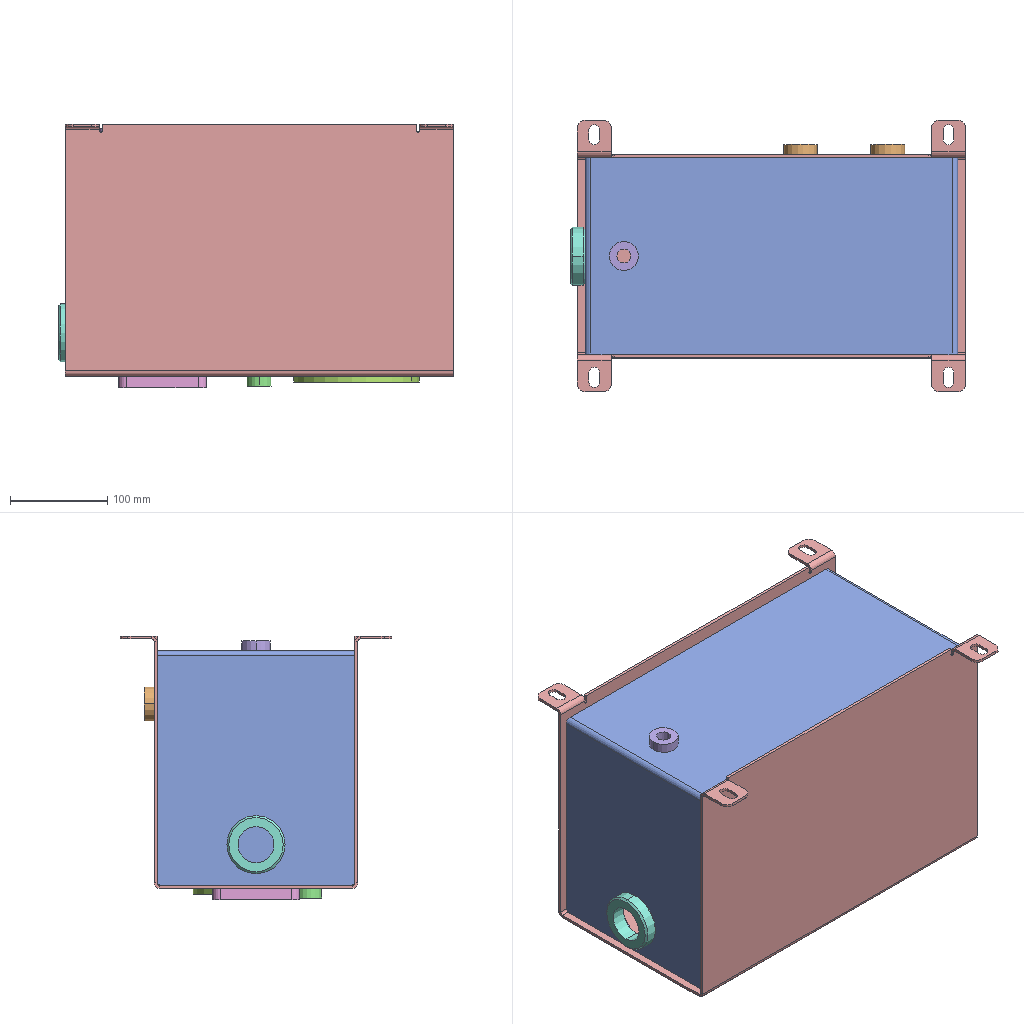Assembly | SolidWorks | 8 different items | 9 placed | box 407 x 280 x 272 mm
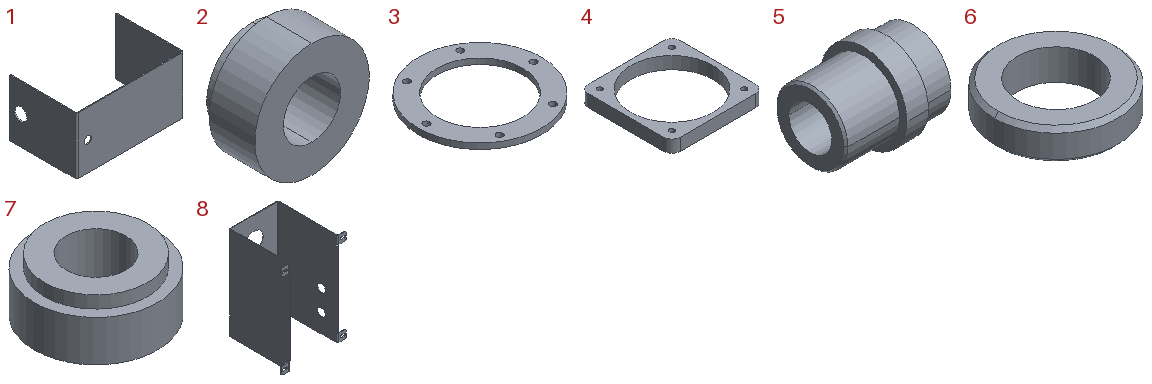Parts list (item | quantity | size | volume | features):
1 | x1 | 384 x 242 x 204 mm | 519134 mm3 | features ICE 2, Fillet 1, FlatPattern 1, SMBaseFlange 1, SheetMetal 1, UnFold 1
2 | x1 | 25 x 13 x 25 mm | 4256 mm3 | features HoleWzd 1, Revolution 1
3 | x1 | 130 x 130 x 6 mm | 40162 mm3 | features FlatPattern 1, HoleWzd 1, SMBaseFlange 1, SheetMetal 1
4 | x1 | 90 x 90 x 12 mm | 35280 mm3 | features FlatPattern 1, HoleWzd 1, SMBaseFlange 1, SheetMetal 1
5 | x2 | 48 x 40 x 40 mm | 30975 mm3 | features HoleWzd 1, ICE 1, Revolution 1
6 | x1 | 60 x 60 x 15 mm | 25107 mm3 | features Chamfer 1, Extrusion 1, HoleWzd 1, ICE 1
7 | x1 | 30 x 30 x 13 mm | 6395 mm3 | features ICE 2, Extrusion 1, HoleWzd 1
8 | x1 | 280 x 260 x 400 mm | 833549 mm3 | features ICE 4, EdgeFlange 1, Fillet 1, FlatPattern 1, SMBaseFlange 1, SheetMetal 1, UnFold 1
Mates (type | each side: item.copy, entity, surface, feature):
Coincident | 8.1 face plane Base-Flange1 | 1.1 face plane Base-Flange1 | 2 times
DistanceDim | 1.1 face plane Base-Flange1 | 8.1 face plane Base-Flange1
Concentric | 8.1 face cylinder Cut-Extrude1 | 3.1 face cylinder Base-Flange1
Coincident | 8.1 face plane Base-Flange1 | 3.1 face plane Base-Flange1
Concentric | 8.1 face cylinder Cut-Extrude1 | 3.1 face cylinder M8 Tapped Hole1
Coincident | 8.1 face plane Base-Flange1 | 4.1 face plane Base-Flange1
Concentric | 8.1 face cylinder Cut-Extrude1 | 4.1 face cylinder Base-Flange1
Parallel | 8.1 face plane Base-Flange1 | 4.1 face plane Base-Flange1
Coincident | 1.1 face plane Base-Flange1 | 6.1 face plane Boss-Extrude1
Concentric | 1.1 face cylinder Cut-Extrude1 | 6.1 face cylinder Boss-Extrude1
Concentric | 8.1 face cylinder Cut-Extrude3 | 5.1 face cylinder Revolve1
Coincident | 8.1 face plane Base-Flange1 | 5.1 face plane Revolve1
Concentric | 8.1 face cylinder Cut-Extrude3 | 5.2 face cylinder Revolve1
Coincident | 8.1 face plane Base-Flange1 | 5.2 face plane Revolve1
Coincident | 1.1 face plane Base-Flange1 | 7.1 face plane Boss-Extrude1
Concentric | 1.1 face cylinder Cut-Extrude2 | 7.1 face cylinder Boss-Extrude1
Concentric | 8.1 edge | 2.1 face cylinder Revolve1
Coincident | 8.1 face plane Base-Flange1 | 2.1 face plane Revolve1